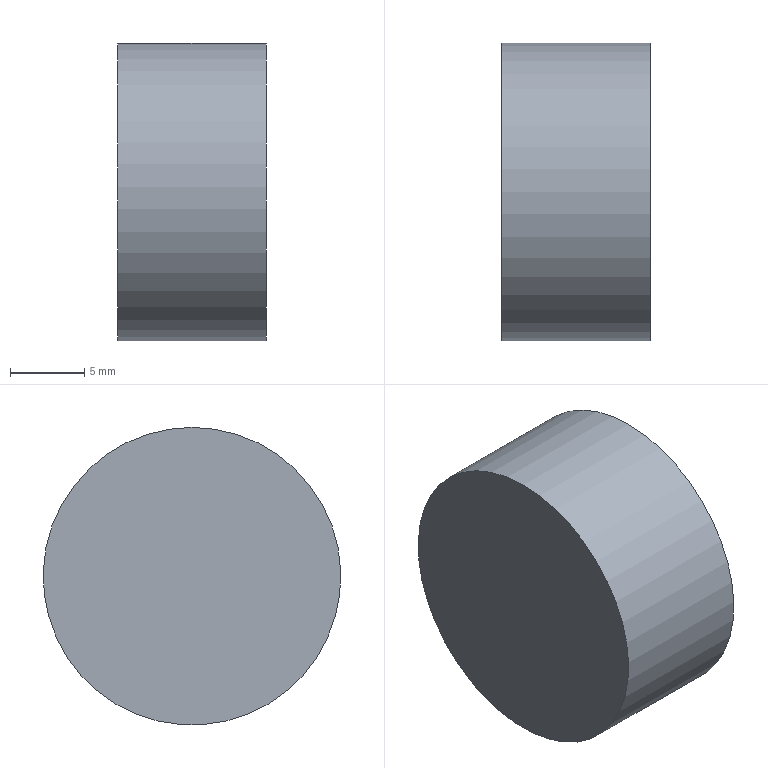Part | NX | features solid 2 | 1 solid | 3 faces | box 10 x 20 x 20 mm | volume 3142 mm3 | plane 2 | cylinder 1 | commonest cylinder face diameters 20 x1
STEP:
#1=CARTESIAN_POINT('',(-1517.9,-440.,-290.));
#2=VERTEX_POINT('',#1);
#3=CARTESIAN_POINT('',(-1517.9,-440.,-300.));
#4=DIRECTION('',(1.,0.,0.));
#5=DIRECTION('',(0.,0.,1.));
#6=AXIS2_PLACEMENT_3D('',#3,#4,#5);
#7=CIRCLE('',#6,10.);
#8=EDGE_CURVE('',#2,#2,#7,.T.);
#9=ORIENTED_EDGE('',*,*,#8,.T.);
#10=EDGE_LOOP('',(#9));
#11=FACE_BOUND('',#10,.T.);
#12=CARTESIAN_POINT('',(-1507.9,-440.,-290.));
#13=VERTEX_POINT('',#12);
#14=CARTESIAN_POINT('',(-1507.9,-440.,-300.));
#15=DIRECTION('',(1.,0.,0.));
#16=DIRECTION('',(0.,0.,1.));
#17=AXIS2_PLACEMENT_3D('',#14,#15,#16);
#18=CIRCLE('',#17,10.);
#19=EDGE_CURVE('',#13,#13,#18,.T.);
#20=ORIENTED_EDGE('',*,*,#19,.F.);
#21=EDGE_LOOP('',(#20));
#22=FACE_BOUND('',#21,.T.);
#23=CARTESIAN_POINT('',(-1503.4,-440.,-300.));
#24=DIRECTION('',(1.,0.,0.));
#25=DIRECTION('',(0.,0.,-1.));
#26=AXIS2_PLACEMENT_3D('',#23,#24,#25);
#27=CYLINDRICAL_SURFACE('',#26,10.);
#28=ADVANCED_FACE('',(#11,#22),#27,.T.);
#29=ORIENTED_EDGE('',*,*,#8,.F.);
#30=EDGE_LOOP('',(#29));
#31=FACE_BOUND('',#30,.T.);
#32=CARTESIAN_POINT('',(-1517.9,-444.5,-300.));
#33=DIRECTION('',(-1.,0.,0.));
#34=DIRECTION('',(0.,0.,1.));
#35=AXIS2_PLACEMENT_3D('',#32,#33,#34);
#36=PLANE('',#35);
#37=ADVANCED_FACE('',(#31),#36,.T.);
#38=ORIENTED_EDGE('',*,*,#19,.T.);
#39=EDGE_LOOP('',(#38));
#40=FACE_BOUND('',#39,.T.);
#41=CARTESIAN_POINT('',(-1507.9,-444.5,-300.));
#42=DIRECTION('',(-1.,0.,0.));
#43=DIRECTION('',(0.,0.,1.));
#44=AXIS2_PLACEMENT_3D('',#41,#42,#43);
#45=PLANE('',#44);
#46=ADVANCED_FACE('',(#40),#45,.F.);
#47=CLOSED_SHELL('',(#28,#37,#46));
#48=MANIFOLD_SOLID_BREP('',#47);
#49=(LENGTH_UNIT()NAMED_UNIT(*)SI_UNIT(.MILLI.,.METRE.));
#50=UNCERTAINTY_MEASURE_WITH_UNIT(LENGTH_MEASURE(0.00001),#49,'','');
#51=(NAMED_UNIT(*)PLANE_ANGLE_UNIT()SI_UNIT($,.RADIAN.));
#52=(NAMED_UNIT(*)SI_UNIT($,.STERADIAN.)SOLID_ANGLE_UNIT());
#53=(GEOMETRIC_REPRESENTATION_CONTEXT(3)GLOBAL_UNCERTAINTY_ASSIGNED_CONTEXT((#50))GLOBAL_UNIT_ASSIGNED_CONTEXT((#49,#51,#52))REPRESENTATION_CONTEXT('',''));
#54=ADVANCED_BREP_SHAPE_REPRESENTATION('',(#48),#53);